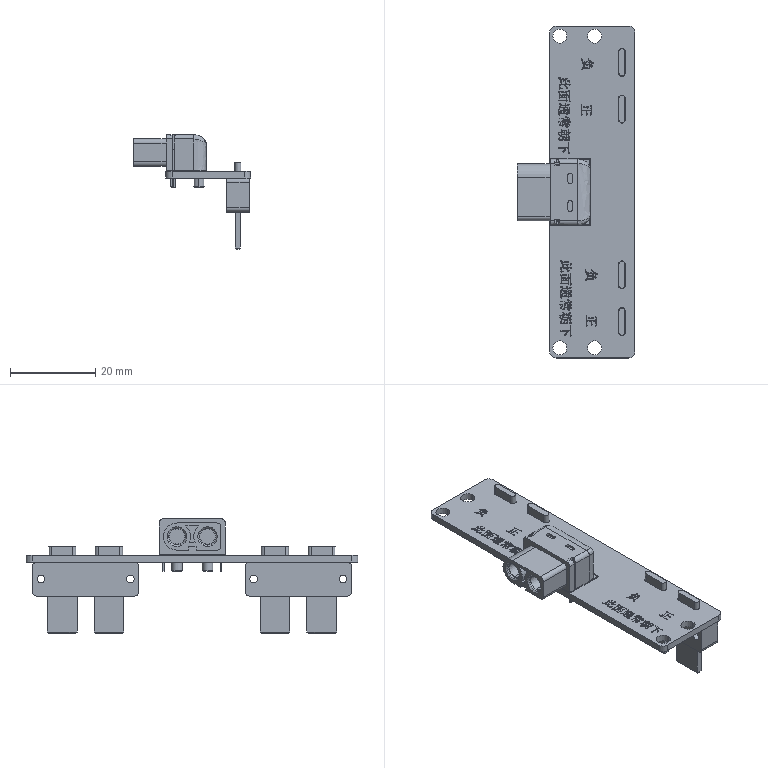Part | SolidWorks | 6 solids | 414 faces | box 27.581 x 78.075 x 26.95 mm | volume 6505 mm3 | plane 287 | cylinder 100 | spline 19 | cone 8 | commonest cylinder face diameters 0.4 x16 2 x14 0.8 x8 1.4 x8 1.6 x8 1.8 x8